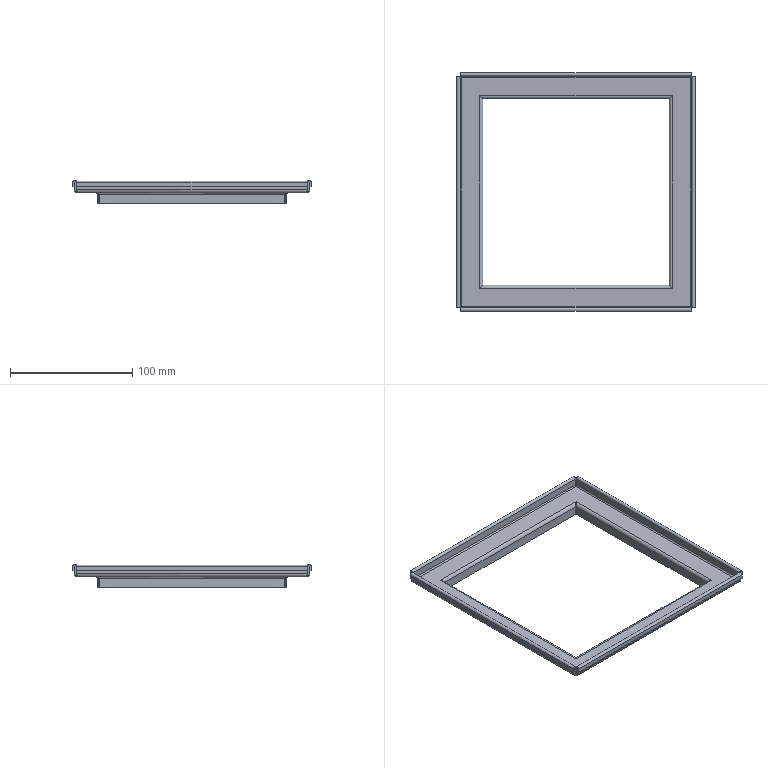Part | SolidWorks | features BaseBody 1 | 1 solid | 106 faces | box 195.2 x 195.2 x 18.5 mm | volume 41385 mm3 | plane 66 | cylinder 24 | spline 16 | commonest cylinder face diameters 2 x8 5 x8 0.1 x4 3.1 x4